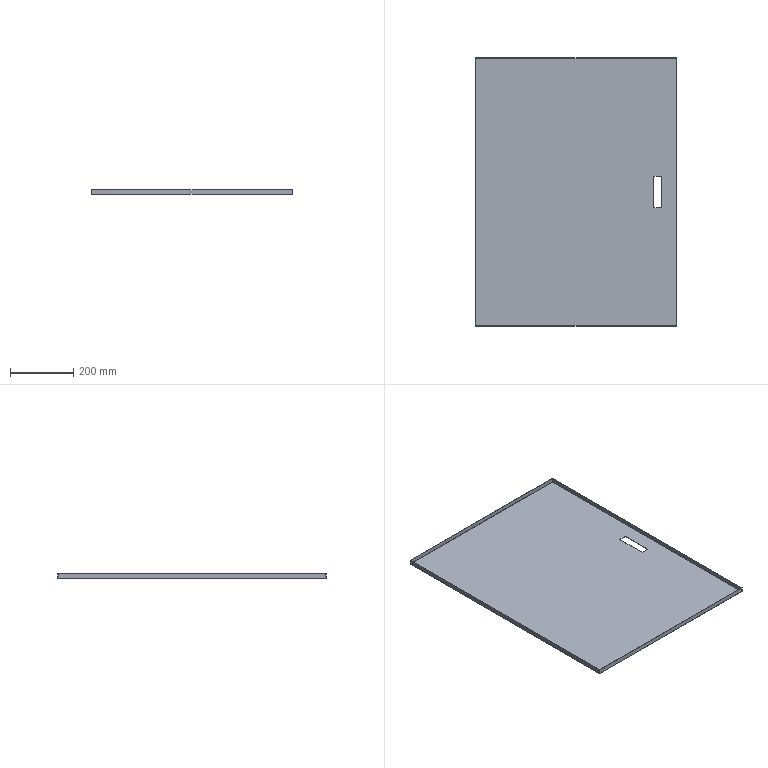Part | STEP file | PN_0010 | 1 solid | 15 faces | box 636 x 850 x 15 mm | volume 579652 mm3 | plane 15
STEP:
#1=CARTESIAN_POINT('',(0.,0.,0.));
#2=DIRECTION('',(0.,0.,1.));
#3=DIRECTION('',(1.,0.,0.));
#4=AXIS2_PLACEMENT_3D('',#1,#2,#3);
#5=CARTESIAN_POINT('',(-318.,425.,0.));
#6=VERTEX_POINT('',#5);
#7=CARTESIAN_POINT('',(-318.,-425.,0.));
#8=VERTEX_POINT('',#7);
#9=CARTESIAN_POINT('',(-318.,-425.,0.));
#10=DIRECTION('',(0.,-1.,0.));
#11=VECTOR('',#10,1.);
#12=LINE('',#9,#11);
#13=CARTESIAN_POINT('',(-318.,-425.,15.));
#14=DIRECTION('',(1.,0.,0.));
#15=DIRECTION('',(0.,0.,-1.));
#16=AXIS2_PLACEMENT_3D('',#13,#14,#15);
#17=PLANE('',#16);
#18=CARTESIAN_POINT('',(15.,0.));
#19=DIRECTION('',(0.,-1.));
#20=VECTOR('',#19,1.);
#21=LINE('',#18,#20);
#22=(GEOMETRIC_REPRESENTATION_CONTEXT(2)PARAMETRIC_REPRESENTATION_CONTEXT()REPRESENTATION_CONTEXT('',''));
#23=DEFINITIONAL_REPRESENTATION('',(#21),#22);
#24=PCURVE('',#17,#23);
#25=CARTESIAN_POINT('',(0.,0.,0.));
#26=DIRECTION('',(0.,0.,1.));
#27=DIRECTION('',(1.,0.,0.));
#28=AXIS2_PLACEMENT_3D('',#25,#26,#27);
#29=PLANE('',#28);
#30=CARTESIAN_POINT('',(-318.,-425.));
#31=DIRECTION('',(0.,-1.));
#32=VECTOR('',#31,1.);
#33=LINE('',#30,#32);
#34=(GEOMETRIC_REPRESENTATION_CONTEXT(2)PARAMETRIC_REPRESENTATION_CONTEXT()REPRESENTATION_CONTEXT('',''));
#35=DEFINITIONAL_REPRESENTATION('',(#33),#34);
#36=PCURVE('',#29,#35);
#37=SURFACE_CURVE('',#12,(#24,#36),.PCURVE_S1.);
#38=EDGE_CURVE('',#6,#8,#37,.T.);
#39=ORIENTED_EDGE('',*,*,#38,.T.);
#40=CARTESIAN_POINT('',(-318.,-425.,15.));
#41=VERTEX_POINT('',#40);
#42=CARTESIAN_POINT('',(-318.,-425.,15.));
#43=DIRECTION('',(0.,0.,-1.));
#44=VECTOR('',#43,1.);
#45=LINE('',#42,#44);
#46=CARTESIAN_POINT('',(0.,0.));
#47=DIRECTION('',(1.,0.));
#48=VECTOR('',#47,1.);
#49=LINE('',#46,#48);
#50=(GEOMETRIC_REPRESENTATION_CONTEXT(2)PARAMETRIC_REPRESENTATION_CONTEXT()REPRESENTATION_CONTEXT('',''));
#51=DEFINITIONAL_REPRESENTATION('',(#49),#50);
#52=PCURVE('',#17,#51);
#53=CARTESIAN_POINT('',(318.,-425.,15.));
#54=DIRECTION('',(0.,1.,0.));
#55=DIRECTION('',(-1.,0.,0.));
#56=AXIS2_PLACEMENT_3D('',#53,#54,#55);
#57=PLANE('',#56);
#58=CARTESIAN_POINT('',(636.,0.));
#59=DIRECTION('',(0.,-1.));
#60=VECTOR('',#59,1.);
#61=LINE('',#58,#60);
#62=(GEOMETRIC_REPRESENTATION_CONTEXT(2)PARAMETRIC_REPRESENTATION_CONTEXT()REPRESENTATION_CONTEXT('',''));
#63=DEFINITIONAL_REPRESENTATION('',(#61),#62);
#64=PCURVE('',#57,#63);
#65=SURFACE_CURVE('',#45,(#52,#64),.PCURVE_S1.);
#66=EDGE_CURVE('',#41,#8,#65,.T.);
#67=ORIENTED_EDGE('',*,*,#66,.F.);
#68=CARTESIAN_POINT('',(-318.,425.,15.));
#69=VERTEX_POINT('',#68);
#70=CARTESIAN_POINT('',(-318.,-425.,15.));
#71=DIRECTION('',(0.,-1.,0.));
#72=VECTOR('',#71,1.);
#73=LINE('',#70,#72);
#74=CARTESIAN_POINT('',(0.,0.));
#75=DIRECTION('',(0.,-1.));
#76=VECTOR('',#75,1.);
#77=LINE('',#74,#76);
#78=(GEOMETRIC_REPRESENTATION_CONTEXT(2)PARAMETRIC_REPRESENTATION_CONTEXT()REPRESENTATION_CONTEXT('',''));
#79=DEFINITIONAL_REPRESENTATION('',(#77),#78);
#80=PCURVE('',#17,#79);
#81=CARTESIAN_POINT('',(0.,0.,15.));
#82=DIRECTION('',(0.,0.,1.));
#83=DIRECTION('',(1.,0.,0.));
#84=AXIS2_PLACEMENT_3D('',#81,#82,#83);
#85=PLANE('',#84);
#86=CARTESIAN_POINT('',(-318.,-425.));
#87=DIRECTION('',(0.,-1.));
#88=VECTOR('',#87,1.);
#89=LINE('',#86,#88);
#90=(GEOMETRIC_REPRESENTATION_CONTEXT(2)PARAMETRIC_REPRESENTATION_CONTEXT()REPRESENTATION_CONTEXT('',''));
#91=DEFINITIONAL_REPRESENTATION('',(#89),#90);
#92=PCURVE('',#85,#91);
#93=SURFACE_CURVE('',#73,(#80,#92),.PCURVE_S1.);
#94=EDGE_CURVE('',#69,#41,#93,.T.);
#95=ORIENTED_EDGE('',*,*,#94,.F.);
#96=CARTESIAN_POINT('',(-318.,425.,15.));
#97=DIRECTION('',(0.,0.,-1.));
#98=VECTOR('',#97,1.);
#99=LINE('',#96,#98);
#100=CARTESIAN_POINT('',(0.,850.));
#101=DIRECTION('',(1.,0.));
#102=VECTOR('',#101,1.);
#103=LINE('',#100,#102);
#104=(GEOMETRIC_REPRESENTATION_CONTEXT(2)PARAMETRIC_REPRESENTATION_CONTEXT()REPRESENTATION_CONTEXT('',''));
#105=DEFINITIONAL_REPRESENTATION('',(#103),#104);
#106=PCURVE('',#17,#105);
#107=CARTESIAN_POINT('',(318.,425.,15.));
#108=DIRECTION('',(0.,-1.,0.));
#109=DIRECTION('',(1.,0.,0.));
#110=AXIS2_PLACEMENT_3D('',#107,#108,#109);
#111=PLANE('',#110);
#112=CARTESIAN_POINT('',(-636.,0.));
#113=DIRECTION('',(0.,-1.));
#114=VECTOR('',#113,1.);
#115=LINE('',#112,#114);
#116=(GEOMETRIC_REPRESENTATION_CONTEXT(2)PARAMETRIC_REPRESENTATION_CONTEXT()REPRESENTATION_CONTEXT('',''));
#117=DEFINITIONAL_REPRESENTATION('',(#115),#116);
#118=PCURVE('',#111,#117);
#119=SURFACE_CURVE('',#99,(#106,#118),.PCURVE_S1.);
#120=EDGE_CURVE('',#69,#6,#119,.T.);
#121=ORIENTED_EDGE('',*,*,#120,.T.);
#122=EDGE_LOOP('',(#39,#67,#95,#121));
#123=FACE_BOUND('',#122,.T.);
#124=ADVANCED_FACE('',(#123),#17,.F.);
#125=CARTESIAN_POINT('',(318.,-425.,0.));
#126=VERTEX_POINT('',#125);
#127=CARTESIAN_POINT('',(318.,-425.,0.));
#128=DIRECTION('',(1.,0.,0.));
#129=VECTOR('',#128,1.);
#130=LINE('',#127,#129);
#131=CARTESIAN_POINT('',(0.,-15.));
#132=DIRECTION('',(-1.,0.));
#133=VECTOR('',#132,1.);
#134=LINE('',#131,#133);
#135=(GEOMETRIC_REPRESENTATION_CONTEXT(2)PARAMETRIC_REPRESENTATION_CONTEXT()REPRESENTATION_CONTEXT('',''));
#136=DEFINITIONAL_REPRESENTATION('',(#134),#135);
#137=PCURVE('',#57,#136);
#138=CARTESIAN_POINT('',(318.,-425.));
#139=DIRECTION('',(1.,0.));
#140=VECTOR('',#139,1.);
#141=LINE('',#138,#140);
#142=(GEOMETRIC_REPRESENTATION_CONTEXT(2)PARAMETRIC_REPRESENTATION_CONTEXT()REPRESENTATION_CONTEXT('',''));
#143=DEFINITIONAL_REPRESENTATION('',(#141),#142);
#144=PCURVE('',#29,#143);
#145=SURFACE_CURVE('',#130,(#137,#144),.PCURVE_S1.);
#146=EDGE_CURVE('',#8,#126,#145,.T.);
#147=ORIENTED_EDGE('',*,*,#146,.T.);
#148=CARTESIAN_POINT('',(318.,-425.,15.));
#149=VERTEX_POINT('',#148);
#150=CARTESIAN_POINT('',(318.,-425.,15.));
#151=DIRECTION('',(0.,0.,-1.));
#152=VECTOR('',#151,1.);
#153=LINE('',#150,#152);
#154=CARTESIAN_POINT('',(0.,0.));
#155=DIRECTION('',(0.,-1.));
#156=VECTOR('',#155,1.);
#157=LINE('',#154,#156);
#158=(GEOMETRIC_REPRESENTATION_CONTEXT(2)PARAMETRIC_REPRESENTATION_CONTEXT()REPRESENTATION_CONTEXT('',''));
#159=DEFINITIONAL_REPRESENTATION('',(#157),#158);
#160=PCURVE('',#57,#159);
#161=CARTESIAN_POINT('',(318.,-425.,15.));
#162=DIRECTION('',(-1.,0.,0.));
#163=DIRECTION('',(0.,0.,1.));
#164=AXIS2_PLACEMENT_3D('',#161,#162,#163);
#165=PLANE('',#164);
#166=CARTESIAN_POINT('',(0.,0.));
#167=DIRECTION('',(-1.,0.));
#168=VECTOR('',#167,1.);
#169=LINE('',#166,#168);
#170=(GEOMETRIC_REPRESENTATION_CONTEXT(2)PARAMETRIC_REPRESENTATION_CONTEXT()REPRESENTATION_CONTEXT('',''));
#171=DEFINITIONAL_REPRESENTATION('',(#169),#170);
#172=PCURVE('',#165,#171);
#173=SURFACE_CURVE('',#153,(#160,#172),.PCURVE_S1.);
#174=EDGE_CURVE('',#149,#126,#173,.T.);
#175=ORIENTED_EDGE('',*,*,#174,.F.);
#176=CARTESIAN_POINT('',(318.,-425.,15.));
#177=DIRECTION('',(1.,0.,0.));
#178=VECTOR('',#177,1.);
#179=LINE('',#176,#178);
#180=CARTESIAN_POINT('',(0.,0.));
#181=DIRECTION('',(-1.,0.));
#182=VECTOR('',#181,1.);
#183=LINE('',#180,#182);
#184=(GEOMETRIC_REPRESENTATION_CONTEXT(2)PARAMETRIC_REPRESENTATION_CONTEXT()REPRESENTATION_CONTEXT('',''));
#185=DEFINITIONAL_REPRESENTATION('',(#183),#184);
#186=PCURVE('',#57,#185);
#187=CARTESIAN_POINT('',(318.,-425.));
#188=DIRECTION('',(1.,0.));
#189=VECTOR('',#188,1.);
#190=LINE('',#187,#189);
#191=(GEOMETRIC_REPRESENTATION_CONTEXT(2)PARAMETRIC_REPRESENTATION_CONTEXT()REPRESENTATION_CONTEXT('',''));
#192=DEFINITIONAL_REPRESENTATION('',(#190),#191);
#193=PCURVE('',#85,#192);
#194=SURFACE_CURVE('',#179,(#186,#193),.PCURVE_S1.);
#195=EDGE_CURVE('',#41,#149,#194,.T.);
#196=ORIENTED_EDGE('',*,*,#195,.F.);
#197=ORIENTED_EDGE('',*,*,#66,.T.);
#198=EDGE_LOOP('',(#147,#175,#196,#197));
#199=FACE_BOUND('',#198,.T.);
#200=ADVANCED_FACE('',(#199),#57,.F.);
#201=CARTESIAN_POINT('',(318.,425.,0.));
#202=VERTEX_POINT('',#201);
#203=CARTESIAN_POINT('',(318.,-425.,0.));
#204=DIRECTION('',(0.,1.,0.));
#205=VECTOR('',#204,1.);
#206=LINE('',#203,#205);
#207=CARTESIAN_POINT('',(-15.,0.));
#208=DIRECTION('',(0.,1.));
#209=VECTOR('',#208,1.);
#210=LINE('',#207,#209);
#211=(GEOMETRIC_REPRESENTATION_CONTEXT(2)PARAMETRIC_REPRESENTATION_CONTEXT()REPRESENTATION_CONTEXT('',''));
#212=DEFINITIONAL_REPRESENTATION('',(#210),#211);
#213=PCURVE('',#165,#212);
#214=CARTESIAN_POINT('',(318.,-425.));
#215=DIRECTION('',(0.,1.));
#216=VECTOR('',#215,1.);
#217=LINE('',#214,#216);
#218=(GEOMETRIC_REPRESENTATION_CONTEXT(2)PARAMETRIC_REPRESENTATION_CONTEXT()REPRESENTATION_CONTEXT('',''));
#219=DEFINITIONAL_REPRESENTATION('',(#217),#218);
#220=PCURVE('',#29,#219);
#221=SURFACE_CURVE('',#206,(#213,#220),.PCURVE_S1.);
#222=EDGE_CURVE('',#126,#202,#221,.T.);
#223=ORIENTED_EDGE('',*,*,#222,.T.);
#224=CARTESIAN_POINT('',(318.,425.,15.));
#225=VERTEX_POINT('',#224);
#226=CARTESIAN_POINT('',(318.,425.,15.));
#227=DIRECTION('',(0.,0.,-1.));
#228=VECTOR('',#227,1.);
#229=LINE('',#226,#228);
#230=CARTESIAN_POINT('',(0.,850.));
#231=DIRECTION('',(-1.,0.));
#232=VECTOR('',#231,1.);
#233=LINE('',#230,#232);
#234=(GEOMETRIC_REPRESENTATION_CONTEXT(2)PARAMETRIC_REPRESENTATION_CONTEXT()REPRESENTATION_CONTEXT('',''));
#235=DEFINITIONAL_REPRESENTATION('',(#233),#234);
#236=PCURVE('',#165,#235);
#237=CARTESIAN_POINT('',(0.,0.));
#238=DIRECTION('',(0.,-1.));
#239=VECTOR('',#238,1.);
#240=LINE('',#237,#239);
#241=(GEOMETRIC_REPRESENTATION_CONTEXT(2)PARAMETRIC_REPRESENTATION_CONTEXT()REPRESENTATION_CONTEXT('',''));
#242=DEFINITIONAL_REPRESENTATION('',(#240),#241);
#243=PCURVE('',#111,#242);
#244=SURFACE_CURVE('',#229,(#236,#243),.PCURVE_S1.);
#245=EDGE_CURVE('',#225,#202,#244,.T.);
#246=ORIENTED_EDGE('',*,*,#245,.F.);
#247=CARTESIAN_POINT('',(318.,-425.,15.));
#248=DIRECTION('',(0.,1.,0.));
#249=VECTOR('',#248,1.);
#250=LINE('',#247,#249);
#251=CARTESIAN_POINT('',(0.,0.));
#252=DIRECTION('',(0.,1.));
#253=VECTOR('',#252,1.);
#254=LINE('',#251,#253);
#255=(GEOMETRIC_REPRESENTATION_CONTEXT(2)PARAMETRIC_REPRESENTATION_CONTEXT()REPRESENTATION_CONTEXT('',''));
#256=DEFINITIONAL_REPRESENTATION('',(#254),#255);
#257=PCURVE('',#165,#256);
#258=CARTESIAN_POINT('',(318.,-425.));
#259=DIRECTION('',(0.,1.));
#260=VECTOR('',#259,1.);
#261=LINE('',#258,#260);
#262=(GEOMETRIC_REPRESENTATION_CONTEXT(2)PARAMETRIC_REPRESENTATION_CONTEXT()REPRESENTATION_CONTEXT('',''));
#263=DEFINITIONAL_REPRESENTATION('',(#261),#262);
#264=PCURVE('',#85,#263);
#265=SURFACE_CURVE('',#250,(#257,#264),.PCURVE_S1.);
#266=EDGE_CURVE('',#149,#225,#265,.T.);
#267=ORIENTED_EDGE('',*,*,#266,.F.);
#268=ORIENTED_EDGE('',*,*,#174,.T.);
#269=EDGE_LOOP('',(#223,#246,#267,#268));
#270=FACE_BOUND('',#269,.T.);
#271=ADVANCED_FACE('',(#270),#165,.F.);
#272=CARTESIAN_POINT('',(318.,425.,0.));
#273=DIRECTION('',(-1.,0.,0.));
#274=VECTOR('',#273,1.);
#275=LINE('',#272,#274);
#276=CARTESIAN_POINT('',(0.,-15.));
#277=DIRECTION('',(-1.,0.));
#278=VECTOR('',#277,1.);
#279=LINE('',#276,#278);
#280=(GEOMETRIC_REPRESENTATION_CONTEXT(2)PARAMETRIC_REPRESENTATION_CONTEXT()REPRESENTATION_CONTEXT('',''));
#281=DEFINITIONAL_REPRESENTATION('',(#279),#280);
#282=PCURVE('',#111,#281);
#283=CARTESIAN_POINT('',(318.,425.));
#284=DIRECTION('',(-1.,0.));
#285=VECTOR('',#284,1.);
#286=LINE('',#283,#285);
#287=(GEOMETRIC_REPRESENTATION_CONTEXT(2)PARAMETRIC_REPRESENTATION_CONTEXT()REPRESENTATION_CONTEXT('',''));
#288=DEFINITIONAL_REPRESENTATION('',(#286),#287);
#289=PCURVE('',#29,#288);
#290=SURFACE_CURVE('',#275,(#282,#289),.PCURVE_S1.);
#291=EDGE_CURVE('',#202,#6,#290,.T.);
#292=ORIENTED_EDGE('',*,*,#291,.T.);
#293=ORIENTED_EDGE('',*,*,#120,.F.);
#294=CARTESIAN_POINT('',(318.,425.,15.));
#295=DIRECTION('',(-1.,0.,0.));
#296=VECTOR('',#295,1.);
#297=LINE('',#294,#296);
#298=CARTESIAN_POINT('',(0.,0.));
#299=DIRECTION('',(-1.,0.));
#300=VECTOR('',#299,1.);
#301=LINE('',#298,#300);
#302=(GEOMETRIC_REPRESENTATION_CONTEXT(2)PARAMETRIC_REPRESENTATION_CONTEXT()REPRESENTATION_CONTEXT('',''));
#303=DEFINITIONAL_REPRESENTATION('',(#301),#302);
#304=PCURVE('',#111,#303);
#305=CARTESIAN_POINT('',(318.,425.));
#306=DIRECTION('',(-1.,0.));
#307=VECTOR('',#306,1.);
#308=LINE('',#305,#307);
#309=(GEOMETRIC_REPRESENTATION_CONTEXT(2)PARAMETRIC_REPRESENTATION_CONTEXT()REPRESENTATION_CONTEXT('',''));
#310=DEFINITIONAL_REPRESENTATION('',(#308),#309);
#311=PCURVE('',#85,#310);
#312=SURFACE_CURVE('',#297,(#304,#311),.PCURVE_S1.);
#313=EDGE_CURVE('',#225,#69,#312,.T.);
#314=ORIENTED_EDGE('',*,*,#313,.F.);
#315=ORIENTED_EDGE('',*,*,#245,.T.);
#316=EDGE_LOOP('',(#292,#293,#314,#315));
#317=FACE_BOUND('',#316,.T.);
#318=ADVANCED_FACE('',(#317),#111,.F.);
#319=CARTESIAN_POINT('',(-317.,424.,15.));
#320=VERTEX_POINT('',#319);
#321=CARTESIAN_POINT('',(-317.,-424.,15.));
#322=VERTEX_POINT('',#321);
#323=CARTESIAN_POINT('',(-317.,-425.,15.));
#324=DIRECTION('',(0.,-1.,0.));
#325=VECTOR('',#324,1.);
#326=LINE('',#323,#325);
#327=CARTESIAN_POINT('',(-317.,-425.));
#328=DIRECTION('',(0.,-1.));
#329=VECTOR('',#328,1.);
#330=LINE('',#327,#329);
#331=(GEOMETRIC_REPRESENTATION_CONTEXT(2)PARAMETRIC_REPRESENTATION_CONTEXT()REPRESENTATION_CONTEXT('',''));
#332=DEFINITIONAL_REPRESENTATION('',(#330),#331);
#333=PCURVE('',#85,#332);
#334=CARTESIAN_POINT('',(-317.,-425.,15.));
#335=DIRECTION('',(1.,0.,0.));
#336=DIRECTION('',(0.,0.,-1.));
#337=AXIS2_PLACEMENT_3D('',#334,#335,#336);
#338=PLANE('',#337);
#339=CARTESIAN_POINT('',(0.,0.));
#340=DIRECTION('',(0.,-1.));
#341=VECTOR('',#340,1.);
#342=LINE('',#339,#341);
#343=(GEOMETRIC_REPRESENTATION_CONTEXT(2)PARAMETRIC_REPRESENTATION_CONTEXT()REPRESENTATION_CONTEXT('',''));
#344=DEFINITIONAL_REPRESENTATION('',(#342),#343);
#345=PCURVE('',#338,#344);
#346=SURFACE_CURVE('',#326,(#333,#345),.PCURVE_S1.);
#347=EDGE_CURVE('',#320,#322,#346,.T.);
#348=ORIENTED_EDGE('',*,*,#347,.F.);
#349=CARTESIAN_POINT('',(317.,424.,15.));
#350=VERTEX_POINT('',#349);
#351=CARTESIAN_POINT('',(318.,424.,15.));
#352=DIRECTION('',(-1.,0.,0.));
#353=VECTOR('',#352,1.);
#354=LINE('',#351,#353);
#355=CARTESIAN_POINT('',(318.,424.));
#356=DIRECTION('',(-1.,0.));
#357=VECTOR('',#356,1.);
#358=LINE('',#355,#357);
#359=(GEOMETRIC_REPRESENTATION_CONTEXT(2)PARAMETRIC_REPRESENTATION_CONTEXT()REPRESENTATION_CONTEXT('',''));
#360=DEFINITIONAL_REPRESENTATION('',(#358),#359);
#361=PCURVE('',#85,#360);
#362=CARTESIAN_POINT('',(318.,424.,15.));
#363=DIRECTION('',(0.,-1.,0.));
#364=DIRECTION('',(1.,0.,0.));
#365=AXIS2_PLACEMENT_3D('',#362,#363,#364);
#366=PLANE('',#365);
#367=CARTESIAN_POINT('',(0.,0.));
#368=DIRECTION('',(-1.,0.));
#369=VECTOR('',#368,1.);
#370=LINE('',#367,#369);
#371=(GEOMETRIC_REPRESENTATION_CONTEXT(2)PARAMETRIC_REPRESENTATION_CONTEXT()REPRESENTATION_CONTEXT('',''));
#372=DEFINITIONAL_REPRESENTATION('',(#370),#371);
#373=PCURVE('',#366,#372);
#374=SURFACE_CURVE('',#354,(#361,#373),.PCURVE_S1.);
#375=EDGE_CURVE('',#350,#320,#374,.T.);
#376=ORIENTED_EDGE('',*,*,#375,.F.);
#377=CARTESIAN_POINT('',(317.,-424.,15.));
#378=VERTEX_POINT('',#377);
#379=CARTESIAN_POINT('',(317.,-425.,15.));
#380=DIRECTION('',(0.,1.,0.));
#381=VECTOR('',#380,1.);
#382=LINE('',#379,#381);
#383=CARTESIAN_POINT('',(317.,-425.));
#384=DIRECTION('',(0.,1.));
#385=VECTOR('',#384,1.);
#386=LINE('',#383,#385);
#387=(GEOMETRIC_REPRESENTATION_CONTEXT(2)PARAMETRIC_REPRESENTATION_CONTEXT()REPRESENTATION_CONTEXT('',''));
#388=DEFINITIONAL_REPRESENTATION('',(#386),#387);
#389=PCURVE('',#85,#388);
#390=CARTESIAN_POINT('',(317.,-425.,15.));
#391=DIRECTION('',(-1.,0.,0.));
#392=DIRECTION('',(0.,0.,1.));
#393=AXIS2_PLACEMENT_3D('',#390,#391,#392);
#394=PLANE('',#393);
#395=CARTESIAN_POINT('',(0.,0.));
#396=DIRECTION('',(0.,1.));
#397=VECTOR('',#396,1.);
#398=LINE('',#395,#397);
#399=(GEOMETRIC_REPRESENTATION_CONTEXT(2)PARAMETRIC_REPRESENTATION_CONTEXT()REPRESENTATION_CONTEXT('',''));
#400=DEFINITIONAL_REPRESENTATION('',(#398),#399);
#401=PCURVE('',#394,#400);
#402=SURFACE_CURVE('',#382,(#389,#401),.PCURVE_S1.);
#403=EDGE_CURVE('',#378,#350,#402,.T.);
#404=ORIENTED_EDGE('',*,*,#403,.F.);
#405=CARTESIAN_POINT('',(318.,-424.,15.));
#406=DIRECTION('',(1.,0.,0.));
#407=VECTOR('',#406,1.);
#408=LINE('',#405,#407);
#409=CARTESIAN_POINT('',(318.,-424.));
#410=DIRECTION('',(1.,0.));
#411=VECTOR('',#410,1.);
#412=LINE('',#409,#411);
#413=(GEOMETRIC_REPRESENTATION_CONTEXT(2)PARAMETRIC_REPRESENTATION_CONTEXT()REPRESENTATION_CONTEXT('',''));
#414=DEFINITIONAL_REPRESENTATION('',(#412),#413);
#415=PCURVE('',#85,#414);
#416=CARTESIAN_POINT('',(318.,-424.,15.));
#417=DIRECTION('',(0.,1.,0.));
#418=DIRECTION('',(-1.,0.,0.));
#419=AXIS2_PLACEMENT_3D('',#416,#417,#418);
#420=PLANE('',#419);
#421=CARTESIAN_POINT('',(0.,0.));
#422=DIRECTION('',(-1.,0.));
#423=VECTOR('',#422,1.);
#424=LINE('',#421,#423);
#425=(GEOMETRIC_REPRESENTATION_CONTEXT(2)PARAMETRIC_REPRESENTATION_CONTEXT()REPRESENTATION_CONTEXT('',''));
#426=DEFINITIONAL_REPRESENTATION('',(#424),#425);
#427=PCURVE('',#420,#426);
#428=SURFACE_CURVE('',#408,(#415,#427),.PCURVE_S1.);
#429=EDGE_CURVE('',#322,#378,#428,.T.);
#430=ORIENTED_EDGE('',*,*,#429,.F.);
#431=EDGE_LOOP('',(#348,#376,#404,#430));
#432=FACE_BOUND('',#431,.T.);
#433=ORIENTED_EDGE('',*,*,#94,.T.);
#434=ORIENTED_EDGE('',*,*,#195,.T.);
#435=ORIENTED_EDGE('',*,*,#266,.T.);
#436=ORIENTED_EDGE('',*,*,#313,.T.);
#437=EDGE_LOOP('',(#433,#434,#435,#436));
#438=FACE_BOUND('',#437,.T.);
#439=ADVANCED_FACE('',(#432,#438),#85,.T.);
#440=CARTESIAN_POINT('',(246.359,50.,0.));
#441=VERTEX_POINT('',#440);
#442=CARTESIAN_POINT('',(271.359,50.,0.));
#443=VERTEX_POINT('',#442);
#444=CARTESIAN_POINT('',(271.359,50.,0.));
#445=DIRECTION('',(1.,0.,0.));
#446=VECTOR('',#445,1.);
#447=LINE('',#444,#446);
#448=CARTESIAN_POINT('',(271.359,50.));
#449=DIRECTION('',(1.,0.));
#450=VECTOR('',#449,1.);
#451=LINE('',#448,#450);
#452=(GEOMETRIC_REPRESENTATION_CONTEXT(2)PARAMETRIC_REPRESENTATION_CONTEXT()REPRESENTATION_CONTEXT('',''));
#453=DEFINITIONAL_REPRESENTATION('',(#451),#452);
#454=PCURVE('',#29,#453);
#455=CARTESIAN_POINT('',(271.359,50.,15.));
#456=DIRECTION('',(0.,1.,0.));
#457=DIRECTION('',(0.,0.,1.));
#458=AXIS2_PLACEMENT_3D('',#455,#456,#457);
#459=PLANE('',#458);
#460=CARTESIAN_POINT('',(-15.,0.));
#461=DIRECTION('',(0.,1.));
#462=VECTOR('',#461,1.);
#463=LINE('',#460,#462);
#464=(GEOMETRIC_REPRESENTATION_CONTEXT(2)PARAMETRIC_REPRESENTATION_CONTEXT()REPRESENTATION_CONTEXT('',''));
#465=DEFINITIONAL_REPRESENTATION('',(#463),#464);
#466=PCURVE('',#459,#465);
#467=SURFACE_CURVE('',#447,(#454,#466),.PCURVE_S1.);
#468=EDGE_CURVE('',#441,#443,#467,.T.);
#469=ORIENTED_EDGE('',*,*,#468,.F.);
#470=CARTESIAN_POINT('',(246.359,-50.,0.));
#471=VERTEX_POINT('',#470);
#472=CARTESIAN_POINT('',(246.359,50.,0.));
#473=DIRECTION('',(0.,1.,0.));
#474=VECTOR('',#473,1.);
#475=LINE('',#472,#474);
#476=CARTESIAN_POINT('',(246.359,50.));
#477=DIRECTION('',(0.,1.));
#478=VECTOR('',#477,1.);
#479=LINE('',#476,#478);
#480=(GEOMETRIC_REPRESENTATION_CONTEXT(2)PARAMETRIC_REPRESENTATION_CONTEXT()REPRESENTATION_CONTEXT('',''));
#481=DEFINITIONAL_REPRESENTATION('',(#479),#480);
#482=PCURVE('',#29,#481);
#483=CARTESIAN_POINT('',(246.359,50.,15.));
#484=DIRECTION('',(-1.,0.,0.));
#485=DIRECTION('',(0.,0.,1.));
#486=AXIS2_PLACEMENT_3D('',#483,#484,#485);
#487=PLANE('',#486);
#488=CARTESIAN_POINT('',(-15.,0.));
#489=DIRECTION('',(0.,1.));
#490=VECTOR('',#489,1.);
#491=LINE('',#488,#490);
#492=(GEOMETRIC_REPRESENTATION_CONTEXT(2)PARAMETRIC_REPRESENTATION_CONTEXT()REPRESENTATION_CONTEXT('',''));
#493=DEFINITIONAL_REPRESENTATION('',(#491),#492);
#494=PCURVE('',#487,#493);
#495=SURFACE_CURVE('',#475,(#482,#494),.PCURVE_S1.);
#496=EDGE_CURVE('',#471,#441,#495,.T.);
#497=ORIENTED_EDGE('',*,*,#496,.F.);
#498=CARTESIAN_POINT('',(271.359,-50.,0.));
#499=VERTEX_POINT('',#498);
#500=CARTESIAN_POINT('',(271.359,-50.,0.));
#501=DIRECTION('',(-1.,0.,0.));
#502=VECTOR('',#501,1.);
#503=LINE('',#500,#502);
#504=CARTESIAN_POINT('',(271.359,-50.));
#505=DIRECTION('',(-1.,0.));
#506=VECTOR('',#505,1.);
#507=LINE('',#504,#506);
#508=(GEOMETRIC_REPRESENTATION_CONTEXT(2)PARAMETRIC_REPRESENTATION_CONTEXT()REPRESENTATION_CONTEXT('',''));
#509=DEFINITIONAL_REPRESENTATION('',(#507),#508);
#510=PCURVE('',#29,#509);
#511=CARTESIAN_POINT('',(271.359,-50.,15.));
#512=DIRECTION('',(0.,-1.,0.));
#513=DIRECTION('',(0.,0.,-1.));
#514=AXIS2_PLACEMENT_3D('',#511,#512,#513);
#515=PLANE('',#514);
#516=CARTESIAN_POINT('',(15.,0.));
#517=DIRECTION('',(0.,-1.));
#518=VECTOR('',#517,1.);
#519=LINE('',#516,#518);
#520=(GEOMETRIC_REPRESENTATION_CONTEXT(2)PARAMETRIC_REPRESENTATION_CONTEXT()REPRESENTATION_CONTEXT('',''));
#521=DEFINITIONAL_REPRESENTATION('',(#519),#520);
#522=PCURVE('',#515,#521);
#523=SURFACE_CURVE('',#503,(#510,#522),.PCURVE_S1.);
#524=EDGE_CURVE('',#499,#471,#523,.T.);
#525=ORIENTED_EDGE('',*,*,#524,.F.);
#526=CARTESIAN_POINT('',(271.359,50.,0.));
#527=DIRECTION('',(0.,-1.,0.));
#528=VECTOR('',#527,1.);
#529=LINE('',#526,#528);
#530=CARTESIAN_POINT('',(271.359,50.));
#531=DIRECTION('',(0.,-1.));
#532=VECTOR('',#531,1.);
#533=LINE('',#530,#532);
#534=(GEOMETRIC_REPRESENTATION_CONTEXT(2)PARAMETRIC_REPRESENTATION_CONTEXT()REPRESENTATION_CONTEXT('',''));
#535=DEFINITIONAL_REPRESENTATION('',(#533),#534);
#536=PCURVE('',#29,#535);
#537=CARTESIAN_POINT('',(271.359,50.,15.));
#538=DIRECTION('',(1.,0.,0.));
#539=DIRECTION('',(0.,0.,-1.));
#540=AXIS2_PLACEMENT_3D('',#537,#538,#539);
#541=PLANE('',#540);
#542=CARTESIAN_POINT('',(15.,0.));
#543=DIRECTION('',(0.,-1.));
#544=VECTOR('',#543,1.);
#545=LINE('',#542,#544);
#546=(GEOMETRIC_REPRESENTATION_CONTEXT(2)PARAMETRIC_REPRESENTATION_CONTEXT()REPRESENTATION_CONTEXT('',''));
#547=DEFINITIONAL_REPRESENTATION('',(#545),#546);
#548=PCURVE('',#541,#547);
#549=SURFACE_CURVE('',#529,(#536,#548),.PCURVE_S1.);
#550=EDGE_CURVE('',#443,#499,#549,.T.);
#551=ORIENTED_EDGE('',*,*,#550,.F.);
#552=EDGE_LOOP('',(#469,#497,#525,#551));
#553=FACE_BOUND('',#552,.T.);
#554=ORIENTED_EDGE('',*,*,#38,.F.);
#555=ORIENTED_EDGE('',*,*,#291,.F.);
#556=ORIENTED_EDGE('',*,*,#222,.F.);
#557=ORIENTED_EDGE('',*,*,#146,.F.);
#558=EDGE_LOOP('',(#554,#555,#556,#557));
#559=FACE_BOUND('',#558,.T.);
#560=ADVANCED_FACE('',(#553,#559),#29,.F.);
#561=CARTESIAN_POINT('',(-317.,424.,1.));
#562=VERTEX_POINT('',#561);
#563=CARTESIAN_POINT('',(-317.,-424.,1.));
#564=VERTEX_POINT('',#563);
#565=CARTESIAN_POINT('',(-317.,-425.,1.));
#566=DIRECTION('',(0.,-1.,0.));
#567=VECTOR('',#566,1.);
#568=LINE('',#565,#567);
#569=CARTESIAN_POINT('',(14.,0.));
#570=DIRECTION('',(0.,-1.));
#571=VECTOR('',#570,1.);
#572=LINE('',#569,#571);
#573=(GEOMETRIC_REPRESENTATION_CONTEXT(2)PARAMETRIC_REPRESENTATION_CONTEXT()REPRESENTATION_CONTEXT('',''));
#574=DEFINITIONAL_REPRESENTATION('',(#572),#573);
#575=PCURVE('',#338,#574);
#576=CARTESIAN_POINT('',(0.,0.,1.));
#577=DIRECTION('',(0.,0.,1.));
#578=DIRECTION('',(1.,0.,0.));
#579=AXIS2_PLACEMENT_3D('',#576,#577,#578);
#580=PLANE('',#579);
#581=CARTESIAN_POINT('',(-317.,-425.));
#582=DIRECTION('',(0.,-1.));
#583=VECTOR('',#582,1.);
#584=LINE('',#581,#583);
#585=(GEOMETRIC_REPRESENTATION_CONTEXT(2)PARAMETRIC_REPRESENTATION_CONTEXT()REPRESENTATION_CONTEXT('',''));
#586=DEFINITIONAL_REPRESENTATION('',(#584),#585);
#587=PCURVE('',#580,#586);
#588=SURFACE_CURVE('',#568,(#575,#587),.PCURVE_S1.);
#589=EDGE_CURVE('',#562,#564,#588,.T.);
#590=ORIENTED_EDGE('',*,*,#589,.F.);
#591=CARTESIAN_POINT('',(-317.,424.,15.));
#592=DIRECTION('',(0.,0.,-1.));
#593=VECTOR('',#592,1.);
#594=LINE('',#591,#593);
#595=CARTESIAN_POINT('',(0.,849.));
#596=DIRECTION('',(1.,0.));
#597=VECTOR('',#596,1.);
#598=LINE('',#595,#597);
#599=(GEOMETRIC_REPRESENTATION_CONTEXT(2)PARAMETRIC_REPRESENTATION_CONTEXT()REPRESENTATION_CONTEXT('',''));
#600=DEFINITIONAL_REPRESENTATION('',(#598),#599);
#601=PCURVE('',#338,#600);
#602=CARTESIAN_POINT('',(-635.,0.));
#603=DIRECTION('',(0.,-1.));
#604=VECTOR('',#603,1.);
#605=LINE('',#602,#604);
#606=(GEOMETRIC_REPRESENTATION_CONTEXT(2)PARAMETRIC_REPRESENTATION_CONTEXT()REPRESENTATION_CONTEXT('',''));
#607=DEFINITIONAL_REPRESENTATION('',(#605),#606);
#608=PCURVE('',#366,#607);
#609=SURFACE_CURVE('',#594,(#601,#608),.PCURVE_S1.);
#610=EDGE_CURVE('',#320,#562,#609,.T.);
#611=ORIENTED_EDGE('',*,*,#610,.F.);
#612=ORIENTED_EDGE('',*,*,#347,.T.);
#613=CARTESIAN_POINT('',(-317.,-424.,15.));
#614=DIRECTION('',(0.,0.,-1.));
#615=VECTOR('',#614,1.);
#616=LINE('',#613,#615);
#617=CARTESIAN_POINT('',(0.,1.));
#618=DIRECTION('',(1.,0.));
#619=VECTOR('',#618,1.);
#620=LINE('',#617,#619);
#621=(GEOMETRIC_REPRESENTATION_CONTEXT(2)PARAMETRIC_REPRESENTATION_CONTEXT()REPRESENTATION_CONTEXT('',''));
#622=DEFINITIONAL_REPRESENTATION('',(#620),#621);
#623=PCURVE('',#338,#622);
#624=CARTESIAN_POINT('',(635.,0.));
#625=DIRECTION('',(0.,-1.));
#626=VECTOR('',#625,1.);
#627=LINE('',#624,#626);
#628=(GEOMETRIC_REPRESENTATION_CONTEXT(2)PARAMETRIC_REPRESENTATION_CONTEXT()REPRESENTATION_CONTEXT('',''));
#629=DEFINITIONAL_REPRESENTATION('',(#627),#628);
#630=PCURVE('',#420,#629);
#631=SURFACE_CURVE('',#616,(#623,#630),.PCURVE_S1.);
#632=EDGE_CURVE('',#322,#564,#631,.T.);
#633=ORIENTED_EDGE('',*,*,#632,.T.);
#634=EDGE_LOOP('',(#590,#611,#612,#633));
#635=FACE_BOUND('',#634,.T.);
#636=ADVANCED_FACE('',(#635),#338,.T.);
#637=CARTESIAN_POINT('',(317.,-424.,1.));
#638=VERTEX_POINT('',#637);
#639=CARTESIAN_POINT('',(318.,-424.,1.));
#640=DIRECTION('',(1.,0.,0.));
#641=VECTOR('',#640,1.);
#642=LINE('',#639,#641);
#643=CARTESIAN_POINT('',(0.,-14.));
#644=DIRECTION('',(-1.,0.));
#645=VECTOR('',#644,1.);
#646=LINE('',#643,#645);
#647=(GEOMETRIC_REPRESENTATION_CONTEXT(2)PARAMETRIC_REPRESENTATION_CONTEXT()REPRESENTATION_CONTEXT('',''));
#648=DEFINITIONAL_REPRESENTATION('',(#646),#647);
#649=PCURVE('',#420,#648);
#650=CARTESIAN_POINT('',(318.,-424.));
#651=DIRECTION('',(1.,0.));
#652=VECTOR('',#651,1.);
#653=LINE('',#650,#652);
#654=(GEOMETRIC_REPRESENTATION_CONTEXT(2)PARAMETRIC_REPRESENTATION_CONTEXT()REPRESENTATION_CONTEXT('',''));
#655=DEFINITIONAL_REPRESENTATION('',(#653),#654);
#656=PCURVE('',#580,#655);
#657=SURFACE_CURVE('',#642,(#649,#656),.PCURVE_S1.);
#658=EDGE_CURVE('',#564,#638,#657,.T.);
#659=ORIENTED_EDGE('',*,*,#658,.F.);
#660=ORIENTED_EDGE('',*,*,#632,.F.);
#661=ORIENTED_EDGE('',*,*,#429,.T.);
#662=CARTESIAN_POINT('',(317.,-424.,15.));
#663=DIRECTION('',(0.,0.,-1.));
#664=VECTOR('',#663,1.);
#665=LINE('',#662,#664);
#666=CARTESIAN_POINT('',(1.,0.));
#667=DIRECTION('',(0.,-1.));
#668=VECTOR('',#667,1.);
#669=LINE('',#666,#668);
#670=(GEOMETRIC_REPRESENTATION_CONTEXT(2)PARAMETRIC_REPRESENTATION_CONTEXT()REPRESENTATION_CONTEXT('',''));
#671=DEFINITIONAL_REPRESENTATION('',(#669),#670);
#672=PCURVE('',#420,#671);
#673=CARTESIAN_POINT('',(0.,1.));
#674=DIRECTION('',(-1.,0.));
#675=VECTOR('',#674,1.);
#676=LINE('',#673,#675);
#677=(GEOMETRIC_REPRESENTATION_CONTEXT(2)PARAMETRIC_REPRESENTATION_CONTEXT()REPRESENTATION_CONTEXT('',''));
#678=DEFINITIONAL_REPRESENTATION('',(#676),#677);
#679=PCURVE('',#394,#678);
#680=SURFACE_CURVE('',#665,(#672,#679),.PCURVE_S1.);
#681=EDGE_CURVE('',#378,#638,#680,.T.);
#682=ORIENTED_EDGE('',*,*,#681,.T.);
#683=EDGE_LOOP('',(#659,#660,#661,#682));
#684=FACE_BOUND('',#683,.T.);
#685=ADVANCED_FACE('',(#684),#420,.T.);
#686=CARTESIAN_POINT('',(317.,424.,1.));
#687=VERTEX_POINT('',#686);
#688=CARTESIAN_POINT('',(317.,-425.,1.));
#689=DIRECTION('',(0.,1.,0.));
#690=VECTOR('',#689,1.);
#691=LINE('',#688,#690);
#692=CARTESIAN_POINT('',(-14.,0.));
#693=DIRECTION('',(0.,1.));
#694=VECTOR('',#693,1.);
#695=LINE('',#692,#694);
#696=(GEOMETRIC_REPRESENTATION_CONTEXT(2)PARAMETRIC_REPRESENTATION_CONTEXT()REPRESENTATION_CONTEXT('',''));
#697=DEFINITIONAL_REPRESENTATION('',(#695),#696);
#698=PCURVE('',#394,#697);
#699=CARTESIAN_POINT('',(317.,-425.));
#700=DIRECTION('',(0.,1.));
#701=VECTOR('',#700,1.);
#702=LINE('',#699,#701);
#703=(GEOMETRIC_REPRESENTATION_CONTEXT(2)PARAMETRIC_REPRESENTATION_CONTEXT()REPRESENTATION_CONTEXT('',''));
#704=DEFINITIONAL_REPRESENTATION('',(#702),#703);
#705=PCURVE('',#580,#704);
#706=SURFACE_CURVE('',#691,(#698,#705),.PCURVE_S1.);
#707=EDGE_CURVE('',#638,#687,#706,.T.);
#708=ORIENTED_EDGE('',*,*,#707,.F.);
#709=ORIENTED_EDGE('',*,*,#681,.F.);
#710=ORIENTED_EDGE('',*,*,#403,.T.);
#711=CARTESIAN_POINT('',(317.,424.,15.));
#712=DIRECTION('',(0.,0.,-1.));
#713=VECTOR('',#712,1.);
#714=LINE('',#711,#713);
#715=CARTESIAN_POINT('',(0.,849.));
#716=DIRECTION('',(-1.,0.));
#717=VECTOR('',#716,1.);
#718=LINE('',#715,#717);
#719=(GEOMETRIC_REPRESENTATION_CONTEXT(2)PARAMETRIC_REPRESENTATION_CONTEXT()REPRESENTATION_CONTEXT('',''));
#720=DEFINITIONAL_REPRESENTATION('',(#718),#719);
#721=PCURVE('',#394,#720);
#722=CARTESIAN_POINT('',(-1.,0.));
#723=DIRECTION('',(0.,-1.));
#724=VECTOR('',#723,1.);
#725=LINE('',#722,#724);
#726=(GEOMETRIC_REPRESENTATION_CONTEXT(2)PARAMETRIC_REPRESENTATION_CONTEXT()REPRESENTATION_CONTEXT('',''));
#727=DEFINITIONAL_REPRESENTATION('',(#725),#726);
#728=PCURVE('',#366,#727);
#729=SURFACE_CURVE('',#714,(#721,#728),.PCURVE_S1.);
#730=EDGE_CURVE('',#350,#687,#729,.T.);
#731=ORIENTED_EDGE('',*,*,#730,.T.);
#732=EDGE_LOOP('',(#708,#709,#710,#731));
#733=FACE_BOUND('',#732,.T.);
#734=ADVANCED_FACE('',(#733),#394,.T.);
#735=CARTESIAN_POINT('',(318.,424.,1.));
#736=DIRECTION('',(-1.,0.,0.));
#737=VECTOR('',#736,1.);
#738=LINE('',#735,#737);
#739=CARTESIAN_POINT('',(0.,-14.));
#740=DIRECTION('',(-1.,0.));
#741=VECTOR('',#740,1.);
#742=LINE('',#739,#741);
#743=(GEOMETRIC_REPRESENTATION_CONTEXT(2)PARAMETRIC_REPRESENTATION_CONTEXT()REPRESENTATION_CONTEXT('',''));
#744=DEFINITIONAL_REPRESENTATION('',(#742),#743);
#745=PCURVE('',#366,#744);
#746=CARTESIAN_POINT('',(318.,424.));
#747=DIRECTION('',(-1.,0.));
#748=VECTOR('',#747,1.);
#749=LINE('',#746,#748);
#750=(GEOMETRIC_REPRESENTATION_CONTEXT(2)PARAMETRIC_REPRESENTATION_CONTEXT()REPRESENTATION_CONTEXT('',''));
#751=DEFINITIONAL_REPRESENTATION('',(#749),#750);
#752=PCURVE('',#580,#751);
#753=SURFACE_CURVE('',#738,(#745,#752),.PCURVE_S1.);
#754=EDGE_CURVE('',#687,#562,#753,.T.);
#755=ORIENTED_EDGE('',*,*,#754,.F.);
#756=ORIENTED_EDGE('',*,*,#730,.F.);
#757=ORIENTED_EDGE('',*,*,#375,.T.);
#758=ORIENTED_EDGE('',*,*,#610,.T.);
#759=EDGE_LOOP('',(#755,#756,#757,#758));
#760=FACE_BOUND('',#759,.T.);
#761=ADVANCED_FACE('',(#760),#366,.T.);
#762=CARTESIAN_POINT('',(246.359,50.,1.));
#763=VERTEX_POINT('',#762);
#764=CARTESIAN_POINT('',(246.359,-50.,1.));
#765=VERTEX_POINT('',#764);
#766=CARTESIAN_POINT('',(246.359,0.,1.));
#767=DIRECTION('',(0.,-1.,0.));
#768=VECTOR('',#767,1.);
#769=LINE('',#766,#768);
#770=CARTESIAN_POINT('',(246.359,0.));
#771=DIRECTION('',(0.,-1.));
#772=VECTOR('',#771,1.);
#773=LINE('',#770,#772);
#774=(GEOMETRIC_REPRESENTATION_CONTEXT(2)PARAMETRIC_REPRESENTATION_CONTEXT()REPRESENTATION_CONTEXT('',''));
#775=DEFINITIONAL_REPRESENTATION('',(#773),#774);
#776=PCURVE('',#580,#775);
#777=CARTESIAN_POINT('',(-14.,-50.));
#778=DIRECTION('',(0.,-1.));
#779=VECTOR('',#778,1.);
#780=LINE('',#777,#779);
#781=(GEOMETRIC_REPRESENTATION_CONTEXT(2)PARAMETRIC_REPRESENTATION_CONTEXT()REPRESENTATION_CONTEXT('',''));
#782=DEFINITIONAL_REPRESENTATION('',(#780),#781);
#783=PCURVE('',#487,#782);
#784=SURFACE_CURVE('',#769,(#776,#783),.PCURVE_S1.);
#785=EDGE_CURVE('',#763,#765,#784,.T.);
#786=ORIENTED_EDGE('',*,*,#785,.F.);
#787=CARTESIAN_POINT('',(271.359,50.,1.));
#788=VERTEX_POINT('',#787);
#789=CARTESIAN_POINT('',(0.,50.,1.));
#790=DIRECTION('',(-1.,0.,0.));
#791=VECTOR('',#790,1.);
#792=LINE('',#789,#791);
#793=CARTESIAN_POINT('',(0.,50.));
#794=DIRECTION('',(-1.,0.));
#795=VECTOR('',#794,1.);
#796=LINE('',#793,#795);
#797=(GEOMETRIC_REPRESENTATION_CONTEXT(2)PARAMETRIC_REPRESENTATION_CONTEXT()REPRESENTATION_CONTEXT('',''));
#798=DEFINITIONAL_REPRESENTATION('',(#796),#797);
#799=PCURVE('',#580,#798);
#800=CARTESIAN_POINT('',(-14.,-271.359));
#801=DIRECTION('',(0.,-1.));
#802=VECTOR('',#801,1.);
#803=LINE('',#800,#802);
#804=(GEOMETRIC_REPRESENTATION_CONTEXT(2)PARAMETRIC_REPRESENTATION_CONTEXT()REPRESENTATION_CONTEXT('',''));
#805=DEFINITIONAL_REPRESENTATION('',(#803),#804);
#806=PCURVE('',#459,#805);
#807=SURFACE_CURVE('',#792,(#799,#806),.PCURVE_S1.);
#808=EDGE_CURVE('',#788,#763,#807,.T.);
#809=ORIENTED_EDGE('',*,*,#808,.F.);
#810=CARTESIAN_POINT('',(271.359,-50.,1.));
#811=VERTEX_POINT('',#810);
#812=CARTESIAN_POINT('',(271.359,0.,1.));
#813=DIRECTION('',(0.,1.,0.));
#814=VECTOR('',#813,1.);
#815=LINE('',#812,#814);
#816=CARTESIAN_POINT('',(271.359,0.));
#817=DIRECTION('',(0.,1.));
#818=VECTOR('',#817,1.);
#819=LINE('',#816,#818);
#820=(GEOMETRIC_REPRESENTATION_CONTEXT(2)PARAMETRIC_REPRESENTATION_CONTEXT()REPRESENTATION_CONTEXT('',''));
#821=DEFINITIONAL_REPRESENTATION('',(#819),#820);
#822=PCURVE('',#580,#821);
#823=CARTESIAN_POINT('',(14.,-50.));
#824=DIRECTION('',(0.,1.));
#825=VECTOR('',#824,1.);
#826=LINE('',#823,#825);
#827=(GEOMETRIC_REPRESENTATION_CONTEXT(2)PARAMETRIC_REPRESENTATION_CONTEXT()REPRESENTATION_CONTEXT('',''));
#828=DEFINITIONAL_REPRESENTATION('',(#826),#827);
#829=PCURVE('',#541,#828);
#830=SURFACE_CURVE('',#815,(#822,#829),.PCURVE_S1.);
#831=EDGE_CURVE('',#811,#788,#830,.T.);
#832=ORIENTED_EDGE('',*,*,#831,.F.);
#833=CARTESIAN_POINT('',(0.,-50.,1.));
#834=DIRECTION('',(1.,0.,0.));
#835=VECTOR('',#834,1.);
#836=LINE('',#833,#835);
#837=CARTESIAN_POINT('',(0.,-50.));
#838=DIRECTION('',(1.,0.));
#839=VECTOR('',#838,1.);
#840=LINE('',#837,#839);
#841=(GEOMETRIC_REPRESENTATION_CONTEXT(2)PARAMETRIC_REPRESENTATION_CONTEXT()REPRESENTATION_CONTEXT('',''));
#842=DEFINITIONAL_REPRESENTATION('',(#840),#841);
#843=PCURVE('',#580,#842);
#844=CARTESIAN_POINT('',(14.,-271.359));
#845=DIRECTION('',(0.,1.));
#846=VECTOR('',#845,1.);
#847=LINE('',#844,#846);
#848=(GEOMETRIC_REPRESENTATION_CONTEXT(2)PARAMETRIC_REPRESENTATION_CONTEXT()REPRESENTATION_CONTEXT('',''));
#849=DEFINITIONAL_REPRESENTATION('',(#847),#848);
#850=PCURVE('',#515,#849);
#851=SURFACE_CURVE('',#836,(#843,#850),.PCURVE_S1.);
#852=EDGE_CURVE('',#765,#811,#851,.T.);
#853=ORIENTED_EDGE('',*,*,#852,.F.);
#854=EDGE_LOOP('',(#786,#809,#832,#853));
#855=FACE_BOUND('',#854,.T.);
#856=ORIENTED_EDGE('',*,*,#589,.T.);
#857=ORIENTED_EDGE('',*,*,#658,.T.);
#858=ORIENTED_EDGE('',*,*,#707,.T.);
#859=ORIENTED_EDGE('',*,*,#754,.T.);
#860=EDGE_LOOP('',(#856,#857,#858,#859));
#861=FACE_BOUND('',#860,.T.);
#862=ADVANCED_FACE('',(#855,#861),#580,.T.);
#863=ORIENTED_EDGE('',*,*,#785,.T.);
#864=CARTESIAN_POINT('',(246.359,-50.,15.));
#865=DIRECTION('',(0.,0.,-1.));
#866=VECTOR('',#865,1.);
#867=LINE('',#864,#866);
#868=CARTESIAN_POINT('',(0.,-100.));
#869=DIRECTION('',(-1.,0.));
#870=VECTOR('',#869,1.);
#871=LINE('',#868,#870);
#872=(GEOMETRIC_REPRESENTATION_CONTEXT(2)PARAMETRIC_REPRESENTATION_CONTEXT()REPRESENTATION_CONTEXT('',''));
#873=DEFINITIONAL_REPRESENTATION('',(#871),#872);
#874=PCURVE('',#487,#873);
#875=CARTESIAN_POINT('',(0.,-25.));
#876=DIRECTION('',(1.,0.));
#877=VECTOR('',#876,1.);
#878=LINE('',#875,#877);
#879=(GEOMETRIC_REPRESENTATION_CONTEXT(2)PARAMETRIC_REPRESENTATION_CONTEXT()REPRESENTATION_CONTEXT('',''));
#880=DEFINITIONAL_REPRESENTATION('',(#878),#879);
#881=PCURVE('',#515,#880);
#882=SURFACE_CURVE('',#867,(#874,#881),.PCURVE_S1.);
#883=EDGE_CURVE('',#765,#471,#882,.T.);
#884=ORIENTED_EDGE('',*,*,#883,.T.);
#885=ORIENTED_EDGE('',*,*,#496,.T.);
#886=CARTESIAN_POINT('',(246.359,50.,15.));
#887=DIRECTION('',(0.,0.,-1.));
#888=VECTOR('',#887,1.);
#889=LINE('',#886,#888);
#890=CARTESIAN_POINT('',(0.,0.));
#891=DIRECTION('',(-1.,0.));
#892=VECTOR('',#891,1.);
#893=LINE('',#890,#892);
#894=(GEOMETRIC_REPRESENTATION_CONTEXT(2)PARAMETRIC_REPRESENTATION_CONTEXT()REPRESENTATION_CONTEXT('',''));
#895=DEFINITIONAL_REPRESENTATION('',(#893),#894);
#896=PCURVE('',#487,#895);
#897=CARTESIAN_POINT('',(0.,-25.));
#898=DIRECTION('',(-1.,0.));
#899=VECTOR('',#898,1.);
#900=LINE('',#897,#899);
#901=(GEOMETRIC_REPRESENTATION_CONTEXT(2)PARAMETRIC_REPRESENTATION_CONTEXT()REPRESENTATION_CONTEXT('',''));
#902=DEFINITIONAL_REPRESENTATION('',(#900),#901);
#903=PCURVE('',#459,#902);
#904=SURFACE_CURVE('',#889,(#896,#903),.PCURVE_S1.);
#905=EDGE_CURVE('',#763,#441,#904,.T.);
#906=ORIENTED_EDGE('',*,*,#905,.F.);
#907=EDGE_LOOP('',(#863,#884,#885,#906));
#908=FACE_BOUND('',#907,.T.);
#909=ADVANCED_FACE('',(#908),#487,.F.);
#910=ORIENTED_EDGE('',*,*,#852,.T.);
#911=CARTESIAN_POINT('',(271.359,-50.,15.));
#912=DIRECTION('',(0.,0.,-1.));
#913=VECTOR('',#912,1.);
#914=LINE('',#911,#913);
#915=CARTESIAN_POINT('',(0.,0.));
#916=DIRECTION('',(1.,0.));
#917=VECTOR('',#916,1.);
#918=LINE('',#915,#917);
#919=(GEOMETRIC_REPRESENTATION_CONTEXT(2)PARAMETRIC_REPRESENTATION_CONTEXT()REPRESENTATION_CONTEXT('',''));
#920=DEFINITIONAL_REPRESENTATION('',(#918),#919);
#921=PCURVE('',#515,#920);
#922=CARTESIAN_POINT('',(0.,-100.));
#923=DIRECTION('',(1.,0.));
#924=VECTOR('',#923,1.);
#925=LINE('',#922,#924);
#926=(GEOMETRIC_REPRESENTATION_CONTEXT(2)PARAMETRIC_REPRESENTATION_CONTEXT()REPRESENTATION_CONTEXT('',''));
#927=DEFINITIONAL_REPRESENTATION('',(#925),#926);
#928=PCURVE('',#541,#927);
#929=SURFACE_CURVE('',#914,(#921,#928),.PCURVE_S1.);
#930=EDGE_CURVE('',#811,#499,#929,.T.);
#931=ORIENTED_EDGE('',*,*,#930,.T.);
#932=ORIENTED_EDGE('',*,*,#524,.T.);
#933=ORIENTED_EDGE('',*,*,#883,.F.);
#934=EDGE_LOOP('',(#910,#931,#932,#933));
#935=FACE_BOUND('',#934,.T.);
#936=ADVANCED_FACE('',(#935),#515,.F.);
#937=ORIENTED_EDGE('',*,*,#831,.T.);
#938=CARTESIAN_POINT('',(271.359,50.,15.));
#939=DIRECTION('',(0.,0.,-1.));
#940=VECTOR('',#939,1.);
#941=LINE('',#938,#940);
#942=CARTESIAN_POINT('',(0.,0.));
#943=DIRECTION('',(1.,0.));
#944=VECTOR('',#943,1.);
#945=LINE('',#942,#944);
#946=(GEOMETRIC_REPRESENTATION_CONTEXT(2)PARAMETRIC_REPRESENTATION_CONTEXT()REPRESENTATION_CONTEXT('',''));
#947=DEFINITIONAL_REPRESENTATION('',(#945),#946);
#948=PCURVE('',#541,#947);
#949=CARTESIAN_POINT('',(0.,0.));
#950=DIRECTION('',(-1.,0.));
#951=VECTOR('',#950,1.);
#952=LINE('',#949,#951);
#953=(GEOMETRIC_REPRESENTATION_CONTEXT(2)PARAMETRIC_REPRESENTATION_CONTEXT()REPRESENTATION_CONTEXT('',''));
#954=DEFINITIONAL_REPRESENTATION('',(#952),#953);
#955=PCURVE('',#459,#954);
#956=SURFACE_CURVE('',#941,(#948,#955),.PCURVE_S1.);
#957=EDGE_CURVE('',#788,#443,#956,.T.);
#958=ORIENTED_EDGE('',*,*,#957,.T.);
#959=ORIENTED_EDGE('',*,*,#550,.T.);
#960=ORIENTED_EDGE('',*,*,#930,.F.);
#961=EDGE_LOOP('',(#937,#958,#959,#960));
#962=FACE_BOUND('',#961,.T.);
#963=ADVANCED_FACE('',(#962),#541,.F.);
#964=ORIENTED_EDGE('',*,*,#808,.T.);
#965=ORIENTED_EDGE('',*,*,#905,.T.);
#966=ORIENTED_EDGE('',*,*,#468,.T.);
#967=ORIENTED_EDGE('',*,*,#957,.F.);
#968=EDGE_LOOP('',(#964,#965,#966,#967));
#969=FACE_BOUND('',#968,.T.);
#970=ADVANCED_FACE('',(#969),#459,.F.);
#971=CLOSED_SHELL('',(#124,#200,#271,#318,#439,#560,#636,#685,#734,#761,#862,#909,#936,#963,#970));
#972=MANIFOLD_SOLID_BREP('',#971);
#973=(LENGTH_UNIT()NAMED_UNIT(*)SI_UNIT(.MILLI.,.METRE.));
#974=UNCERTAINTY_MEASURE_WITH_UNIT(LENGTH_MEASURE(0.0000001),#973,'','');
#975=(NAMED_UNIT(*)PLANE_ANGLE_UNIT()SI_UNIT($,.RADIAN.));
#976=(NAMED_UNIT(*)SI_UNIT($,.STERADIAN.)SOLID_ANGLE_UNIT());
#977=(GEOMETRIC_REPRESENTATION_CONTEXT(3)GLOBAL_UNCERTAINTY_ASSIGNED_CONTEXT((#974))GLOBAL_UNIT_ASSIGNED_CONTEXT((#973,#975,#976))REPRESENTATION_CONTEXT('',''));
#978=ADVANCED_BREP_SHAPE_REPRESENTATION('',(#4,#972),#977);